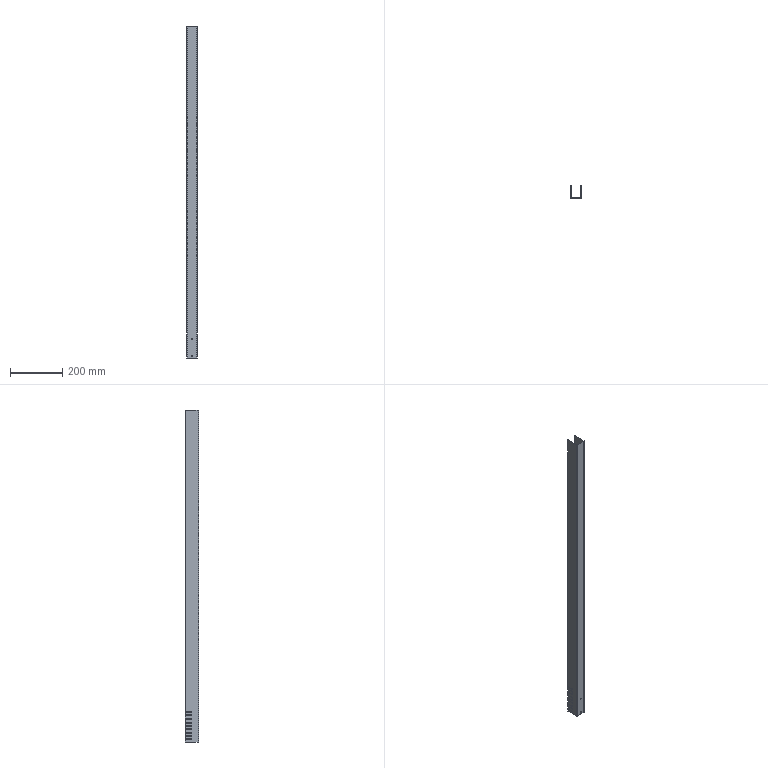Part | SolidWorks | features Cut 1, FlatPattern 1, ICE 1, LPattern 1, SMBaseFlange 1, SheetMetal 1 | 1 solid | 98 faces | box 40 x 50 x 1273 mm | volume 257458 mm3 | plane 90 | cylinder 8 | commonest cylinder face diameters 5 x4 0.4 x2 3.4 x2